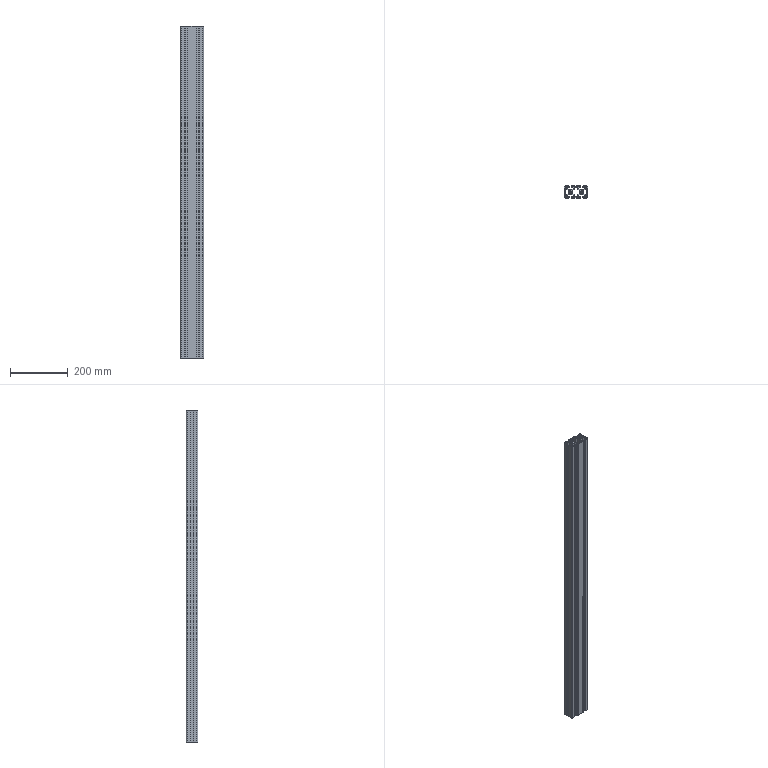Part | STEP file | LE-8-4080W-S-OO_LE0912125351 | 1 solid | 166 faces | box 80 x 40 x 1150 mm | volume 1377772 mm3 | plane 126 | cylinder 40 | commonest cylinder face diameters 0.4 x24 5.9 x8 6.8 x4 7 x4